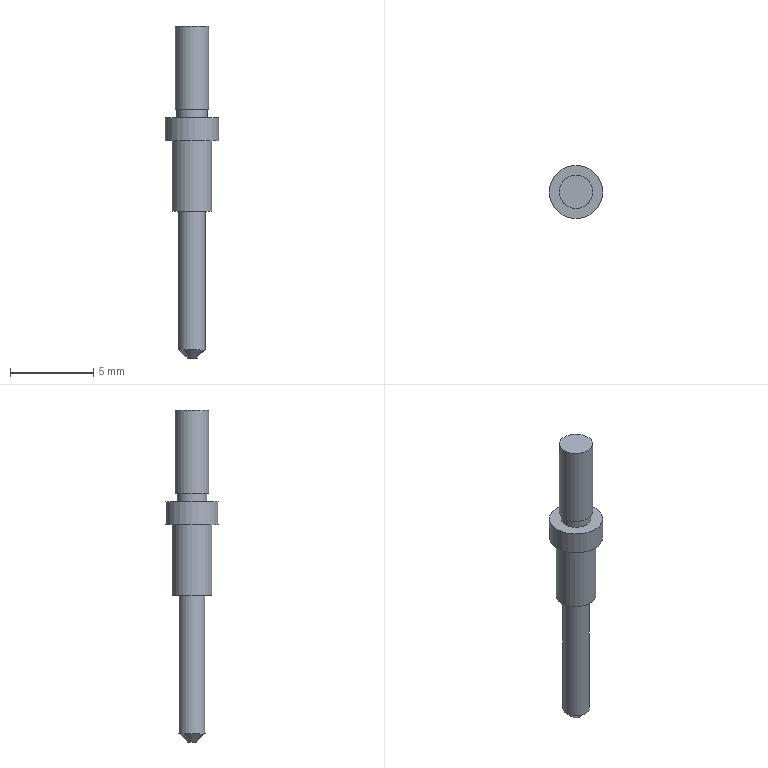Part | STEP file | Radial combiner probe | 1 solid | 12 faces | box 3.2 x 3.2 x 19.92 mm | volume 64.491 mm3 | plane 6 | cylinder 5 | cone 1 | commonest cylinder face diameters 1.6 x1 1.8 x1 2 x1 2.4 x1 3.2 x1
STEP:
#1=CARTESIAN_POINT('',(0.,0.,0.));
#2=DIRECTION('',(0.,0.,1.));
#3=DIRECTION('',(1.,0.,0.));
#4=AXIS2_PLACEMENT_3D('',#1,#2,#3);
#5=CARTESIAN_POINT('',(-216.619,-165.137,75.792));
#6=VERTEX_POINT('',#5);
#7=CARTESIAN_POINT('',(-215.019,-165.137,75.792));
#8=DIRECTION('',(0.,0.,-1.));
#9=DIRECTION('',(-1.,0.,0.));
#10=AXIS2_PLACEMENT_3D('',#7,#8,#9);
#11=CIRCLE('',#10,1.6);
#12=CARTESIAN_POINT('',(-215.019,-165.137,74.402));
#13=DIRECTION('',(0.,0.,1.));
#14=DIRECTION('',(1.,0.,0.));
#15=AXIS2_PLACEMENT_3D('',#12,#13,#14);
#16=CYLINDRICAL_SURFACE('',#15,1.6);
#17=CARTESIAN_POINT('',(9.425,1.39));
#18=DIRECTION('',(-1.,0.));
#19=VECTOR('',#18,1.);
#20=LINE('',#17,#19);
#21=(GEOMETRIC_REPRESENTATION_CONTEXT(2)PARAMETRIC_REPRESENTATION_CONTEXT()REPRESENTATION_CONTEXT('',''));
#22=DEFINITIONAL_REPRESENTATION('',(#20),#21);
#23=PCURVE('',#16,#22);
#24=CARTESIAN_POINT('',(-215.019,-165.137,75.792));
#25=DIRECTION('',(0.,0.,-1.));
#26=DIRECTION('',(-1.,0.,0.));
#27=AXIS2_PLACEMENT_3D('',#24,#25,#26);
#28=PLANE('',#27);
#29=CARTESIAN_POINT('',(0.,0.));
#30=DIRECTION('',(1.,0.));
#31=AXIS2_PLACEMENT_2D('',#29,#30);
#32=CIRCLE('',#31,1.6);
#33=(GEOMETRIC_REPRESENTATION_CONTEXT(2)PARAMETRIC_REPRESENTATION_CONTEXT()REPRESENTATION_CONTEXT('',''));
#34=DEFINITIONAL_REPRESENTATION('',(#32),#33);
#35=PCURVE('',#28,#34);
#36=SURFACE_CURVE('',#11,(#23,#35),.PCURVE_S1.);
#37=EDGE_CURVE('',#6,#6,#36,.T.);
#38=ORIENTED_EDGE('',*,*,#37,.T.);
#39=CARTESIAN_POINT('',(-216.619,-165.137,74.402));
#40=VERTEX_POINT('',#39);
#41=CARTESIAN_POINT('',(-216.619,-165.137,74.402));
#42=CARTESIAN_POINT('',(-216.619,-165.137,75.792));
#43=B_SPLINE_CURVE_WITH_KNOTS('',1,(#41,#42),.UNSPECIFIED.,.F.,.F.,(2,2),(0.,1.39),.PIECEWISE_BEZIER_KNOTS.);
#44=CARTESIAN_POINT('',(3.142,0.));
#45=DIRECTION('',(0.,1.));
#46=VECTOR('',#45,1.);
#47=LINE('',#44,#46);
#48=(GEOMETRIC_REPRESENTATION_CONTEXT(2)PARAMETRIC_REPRESENTATION_CONTEXT()REPRESENTATION_CONTEXT('',''));
#49=DEFINITIONAL_REPRESENTATION('',(#47),#48);
#50=PCURVE('',#16,#49);
#51=CARTESIAN_POINT('',(9.425,0.));
#52=DIRECTION('',(0.,1.));
#53=VECTOR('',#52,1.);
#54=LINE('',#51,#53);
#55=(GEOMETRIC_REPRESENTATION_CONTEXT(2)PARAMETRIC_REPRESENTATION_CONTEXT()REPRESENTATION_CONTEXT('',''));
#56=DEFINITIONAL_REPRESENTATION('',(#54),#55);
#57=PCURVE('',#16,#56);
#58=SEAM_CURVE('',#43,(#50,#57),.PCURVE_S1.);
#59=EDGE_CURVE('',#40,#6,#58,.T.);
#60=ORIENTED_EDGE('',*,*,#59,.F.);
#61=CARTESIAN_POINT('',(-215.019,-165.137,74.402));
#62=DIRECTION('',(0.,0.,-1.));
#63=DIRECTION('',(-1.,0.,0.));
#64=AXIS2_PLACEMENT_3D('',#61,#62,#63);
#65=CIRCLE('',#64,1.6);
#66=CARTESIAN_POINT('',(9.425,0.));
#67=DIRECTION('',(-1.,0.));
#68=VECTOR('',#67,1.);
#69=LINE('',#66,#68);
#70=(GEOMETRIC_REPRESENTATION_CONTEXT(2)PARAMETRIC_REPRESENTATION_CONTEXT()REPRESENTATION_CONTEXT('',''));
#71=DEFINITIONAL_REPRESENTATION('',(#69),#70);
#72=PCURVE('',#16,#71);
#73=CARTESIAN_POINT('',(-215.019,-165.137,74.402));
#74=DIRECTION('',(0.,0.,-1.));
#75=DIRECTION('',(-1.,0.,0.));
#76=AXIS2_PLACEMENT_3D('',#73,#74,#75);
#77=PLANE('',#76);
#78=CARTESIAN_POINT('',(0.,0.));
#79=DIRECTION('',(1.,0.));
#80=AXIS2_PLACEMENT_2D('',#78,#79);
#81=CIRCLE('',#80,1.6);
#82=(GEOMETRIC_REPRESENTATION_CONTEXT(2)PARAMETRIC_REPRESENTATION_CONTEXT()REPRESENTATION_CONTEXT('',''));
#83=DEFINITIONAL_REPRESENTATION('',(#81),#82);
#84=PCURVE('',#77,#83);
#85=SURFACE_CURVE('',#65,(#72,#84),.PCURVE_S1.);
#86=EDGE_CURVE('',#40,#40,#85,.T.);
#87=ORIENTED_EDGE('',*,*,#86,.F.);
#88=ORIENTED_EDGE('',*,*,#59,.T.);
#89=EDGE_LOOP('',(#38,#60,#87,#88));
#90=FACE_BOUND('',#89,.T.);
#91=ADVANCED_FACE('',(#90),#16,.T.);
#92=CARTESIAN_POINT('',(-216.219,-165.137,74.402));
#93=VERTEX_POINT('',#92);
#94=CARTESIAN_POINT('',(-215.019,-165.137,74.402));
#95=DIRECTION('',(0.,0.,-1.));
#96=DIRECTION('',(-1.,0.,0.));
#97=AXIS2_PLACEMENT_3D('',#94,#95,#96);
#98=CIRCLE('',#97,1.2);
#99=CARTESIAN_POINT('',(0.,0.));
#100=DIRECTION('',(1.,0.));
#101=AXIS2_PLACEMENT_2D('',#99,#100);
#102=CIRCLE('',#101,1.2);
#103=(GEOMETRIC_REPRESENTATION_CONTEXT(2)PARAMETRIC_REPRESENTATION_CONTEXT()REPRESENTATION_CONTEXT('',''));
#104=DEFINITIONAL_REPRESENTATION('',(#102),#103);
#105=PCURVE('',#77,#104);
#106=CARTESIAN_POINT('',(-215.019,-165.137,70.172));
#107=DIRECTION('',(0.,0.,1.));
#108=DIRECTION('',(1.,0.,0.));
#109=AXIS2_PLACEMENT_3D('',#106,#107,#108);
#110=CYLINDRICAL_SURFACE('',#109,1.2);
#111=CARTESIAN_POINT('',(9.425,4.23));
#112=DIRECTION('',(-1.,0.));
#113=VECTOR('',#112,1.);
#114=LINE('',#111,#113);
#115=(GEOMETRIC_REPRESENTATION_CONTEXT(2)PARAMETRIC_REPRESENTATION_CONTEXT()REPRESENTATION_CONTEXT('',''));
#116=DEFINITIONAL_REPRESENTATION('',(#114),#115);
#117=PCURVE('',#110,#116);
#118=SURFACE_CURVE('',#98,(#105,#117),.PCURVE_S1.);
#119=EDGE_CURVE('',#93,#93,#118,.T.);
#120=ORIENTED_EDGE('',*,*,#119,.F.);
#121=EDGE_LOOP('',(#120));
#122=FACE_BOUND('',#121,.T.);
#123=ORIENTED_EDGE('',*,*,#86,.T.);
#124=EDGE_LOOP('',(#123));
#125=FACE_BOUND('',#124,.T.);
#126=ADVANCED_FACE('',(#122,#125),#77,.T.);
#127=CARTESIAN_POINT('',(-214.119,-165.137,75.792));
#128=VERTEX_POINT('',#127);
#129=CARTESIAN_POINT('',(-215.019,-165.137,75.792));
#130=DIRECTION('',(0.,0.,1.));
#131=DIRECTION('',(1.,0.,0.));
#132=AXIS2_PLACEMENT_3D('',#129,#130,#131);
#133=CIRCLE('',#132,0.9);
#134=CARTESIAN_POINT('',(-0.9,0.));
#135=CARTESIAN_POINT('',(-0.9,1.559));
#136=CARTESIAN_POINT('',(0.45,0.7794));
#137=CARTESIAN_POINT('',(1.8,0.));
#138=CARTESIAN_POINT('',(0.45,-0.7794));
#139=CARTESIAN_POINT('',(-0.9,-1.559));
#140=CARTESIAN_POINT('',(-0.9,0.));
#141=(BOUNDED_CURVE()B_SPLINE_CURVE(2,(#134,#135,#136,#137,#138,#139,#140),.UNSPECIFIED.,.T.,.F.)B_SPLINE_CURVE_WITH_KNOTS((1,2,2,2,2,1),(-2.094,0.,2.094,4.189,6.283,8.378),.UNSPECIFIED.)CURVE()GEOMETRIC_REPRESENTATION_ITEM()RATIONAL_B_SPLINE_CURVE((1.,0.5,1.,0.5,1.,0.5,1.))REPRESENTATION_ITEM(''));
#142=(GEOMETRIC_REPRESENTATION_CONTEXT(2)PARAMETRIC_REPRESENTATION_CONTEXT()REPRESENTATION_CONTEXT('',''));
#143=DEFINITIONAL_REPRESENTATION('',(#141),#142);
#144=PCURVE('',#28,#143);
#145=CARTESIAN_POINT('',(-215.019,-165.137,76.292));
#146=DIRECTION('',(0.,0.,-1.));
#147=DIRECTION('',(-1.,0.,0.));
#148=AXIS2_PLACEMENT_3D('',#145,#146,#147);
#149=CYLINDRICAL_SURFACE('',#148,0.9);
#150=CARTESIAN_POINT('',(9.425,0.5));
#151=DIRECTION('',(-1.,0.));
#152=VECTOR('',#151,1.);
#153=LINE('',#150,#152);
#154=(GEOMETRIC_REPRESENTATION_CONTEXT(2)PARAMETRIC_REPRESENTATION_CONTEXT()REPRESENTATION_CONTEXT('',''));
#155=DEFINITIONAL_REPRESENTATION('',(#153),#154);
#156=PCURVE('',#149,#155);
#157=SURFACE_CURVE('',#133,(#144,#156),.PCURVE_S1.);
#158=EDGE_CURVE('',#128,#128,#157,.T.);
#159=ORIENTED_EDGE('',*,*,#158,.F.);
#160=EDGE_LOOP('',(#159));
#161=FACE_BOUND('',#160,.T.);
#162=ORIENTED_EDGE('',*,*,#37,.F.);
#163=EDGE_LOOP('',(#162));
#164=FACE_BOUND('',#163,.T.);
#165=ADVANCED_FACE('',(#161,#164),#28,.F.);
#166=ORIENTED_EDGE('',*,*,#119,.T.);
#167=CARTESIAN_POINT('',(-216.219,-165.137,70.172));
#168=VERTEX_POINT('',#167);
#169=CARTESIAN_POINT('',(-216.219,-165.137,70.172));
#170=CARTESIAN_POINT('',(-216.219,-165.137,74.402));
#171=B_SPLINE_CURVE_WITH_KNOTS('',1,(#169,#170),.UNSPECIFIED.,.F.,.F.,(2,2),(0.,4.23),.PIECEWISE_BEZIER_KNOTS.);
#172=CARTESIAN_POINT('',(3.142,0.));
#173=DIRECTION('',(0.,1.));
#174=VECTOR('',#173,1.);
#175=LINE('',#172,#174);
#176=(GEOMETRIC_REPRESENTATION_CONTEXT(2)PARAMETRIC_REPRESENTATION_CONTEXT()REPRESENTATION_CONTEXT('',''));
#177=DEFINITIONAL_REPRESENTATION('',(#175),#176);
#178=PCURVE('',#110,#177);
#179=CARTESIAN_POINT('',(9.425,0.));
#180=DIRECTION('',(0.,1.));
#181=VECTOR('',#180,1.);
#182=LINE('',#179,#181);
#183=(GEOMETRIC_REPRESENTATION_CONTEXT(2)PARAMETRIC_REPRESENTATION_CONTEXT()REPRESENTATION_CONTEXT('',''));
#184=DEFINITIONAL_REPRESENTATION('',(#182),#183);
#185=PCURVE('',#110,#184);
#186=SEAM_CURVE('',#171,(#178,#185),.PCURVE_S1.);
#187=EDGE_CURVE('',#168,#93,#186,.T.);
#188=ORIENTED_EDGE('',*,*,#187,.F.);
#189=CARTESIAN_POINT('',(-215.019,-165.137,70.172));
#190=DIRECTION('',(0.,0.,-1.));
#191=DIRECTION('',(-1.,0.,0.));
#192=AXIS2_PLACEMENT_3D('',#189,#190,#191);
#193=CIRCLE('',#192,1.2);
#194=CARTESIAN_POINT('',(9.425,0.));
#195=DIRECTION('',(-1.,0.));
#196=VECTOR('',#195,1.);
#197=LINE('',#194,#196);
#198=(GEOMETRIC_REPRESENTATION_CONTEXT(2)PARAMETRIC_REPRESENTATION_CONTEXT()REPRESENTATION_CONTEXT('',''));
#199=DEFINITIONAL_REPRESENTATION('',(#197),#198);
#200=PCURVE('',#110,#199);
#201=CARTESIAN_POINT('',(-215.019,-165.137,70.172));
#202=DIRECTION('',(0.,0.,-1.));
#203=DIRECTION('',(-1.,0.,0.));
#204=AXIS2_PLACEMENT_3D('',#201,#202,#203);
#205=PLANE('',#204);
#206=CARTESIAN_POINT('',(0.,0.));
#207=DIRECTION('',(1.,0.));
#208=AXIS2_PLACEMENT_2D('',#206,#207);
#209=CIRCLE('',#208,1.2);
#210=(GEOMETRIC_REPRESENTATION_CONTEXT(2)PARAMETRIC_REPRESENTATION_CONTEXT()REPRESENTATION_CONTEXT('',''));
#211=DEFINITIONAL_REPRESENTATION('',(#209),#210);
#212=PCURVE('',#205,#211);
#213=SURFACE_CURVE('',#193,(#200,#212),.PCURVE_S1.);
#214=EDGE_CURVE('',#168,#168,#213,.T.);
#215=ORIENTED_EDGE('',*,*,#214,.F.);
#216=ORIENTED_EDGE('',*,*,#187,.T.);
#217=EDGE_LOOP('',(#166,#188,#215,#216));
#218=FACE_BOUND('',#217,.T.);
#219=ADVANCED_FACE('',(#218),#110,.T.);
#220=CARTESIAN_POINT('',(-215.819,-165.137,70.172));
#221=VERTEX_POINT('',#220);
#222=CARTESIAN_POINT('',(-215.019,-165.137,70.172));
#223=DIRECTION('',(0.,0.,-1.));
#224=DIRECTION('',(-1.,0.,0.));
#225=AXIS2_PLACEMENT_3D('',#222,#223,#224);
#226=CIRCLE('',#225,0.8);
#227=CARTESIAN_POINT('',(0.,0.));
#228=DIRECTION('',(1.,0.));
#229=AXIS2_PLACEMENT_2D('',#227,#228);
#230=CIRCLE('',#229,0.8);
#231=(GEOMETRIC_REPRESENTATION_CONTEXT(2)PARAMETRIC_REPRESENTATION_CONTEXT()REPRESENTATION_CONTEXT('',''));
#232=DEFINITIONAL_REPRESENTATION('',(#230),#231);
#233=PCURVE('',#205,#232);
#234=CARTESIAN_POINT('',(-215.019,-165.137,61.372));
#235=DIRECTION('',(0.,0.,1.));
#236=DIRECTION('',(1.,0.,0.));
#237=AXIS2_PLACEMENT_3D('',#234,#235,#236);
#238=CYLINDRICAL_SURFACE('',#237,0.8);
#239=CARTESIAN_POINT('',(9.425,8.8));
#240=DIRECTION('',(-1.,0.));
#241=VECTOR('',#240,1.);
#242=LINE('',#239,#241);
#243=(GEOMETRIC_REPRESENTATION_CONTEXT(2)PARAMETRIC_REPRESENTATION_CONTEXT()REPRESENTATION_CONTEXT('',''));
#244=DEFINITIONAL_REPRESENTATION('',(#242),#243);
#245=PCURVE('',#238,#244);
#246=SURFACE_CURVE('',#226,(#233,#245),.PCURVE_S1.);
#247=EDGE_CURVE('',#221,#221,#246,.T.);
#248=ORIENTED_EDGE('',*,*,#247,.F.);
#249=EDGE_LOOP('',(#248));
#250=FACE_BOUND('',#249,.T.);
#251=ORIENTED_EDGE('',*,*,#214,.T.);
#252=EDGE_LOOP('',(#251));
#253=FACE_BOUND('',#252,.T.);
#254=ADVANCED_FACE('',(#250,#253),#205,.T.);
#255=CARTESIAN_POINT('',(-215.819,-165.137,61.872));
#256=VERTEX_POINT('',#255);
#257=CARTESIAN_POINT('',(-215.019,-165.137,61.872));
#258=DIRECTION('',(0.,0.,1.));
#259=DIRECTION('',(-1.,0.,0.));
#260=AXIS2_PLACEMENT_3D('',#257,#258,#259);
#261=CIRCLE('',#260,0.8);
#262=CARTESIAN_POINT('',(3.142,0.5));
#263=DIRECTION('',(1.,0.));
#264=VECTOR('',#263,1.);
#265=LINE('',#262,#264);
#266=(GEOMETRIC_REPRESENTATION_CONTEXT(2)PARAMETRIC_REPRESENTATION_CONTEXT()REPRESENTATION_CONTEXT('',''));
#267=DEFINITIONAL_REPRESENTATION('',(#265),#266);
#268=PCURVE('',#238,#267);
#269=CARTESIAN_POINT('',(-215.019,-165.137,61.372));
#270=DIRECTION('',(0.,0.,1.));
#271=DIRECTION('',(1.,0.,0.));
#272=AXIS2_PLACEMENT_3D('',#269,#270,#271);
#273=CONICAL_SURFACE('',#272,0.3,0.7854);
#274=CARTESIAN_POINT('',(3.142,0.5));
#275=DIRECTION('',(1.,0.));
#276=VECTOR('',#275,1.);
#277=LINE('',#274,#276);
#278=(GEOMETRIC_REPRESENTATION_CONTEXT(2)PARAMETRIC_REPRESENTATION_CONTEXT()REPRESENTATION_CONTEXT('',''));
#279=DEFINITIONAL_REPRESENTATION('',(#277),#278);
#280=PCURVE('',#273,#279);
#281=SURFACE_CURVE('',#261,(#268,#280),.PCURVE_S1.);
#282=EDGE_CURVE('',#256,#256,#281,.T.);
#283=ORIENTED_EDGE('',*,*,#282,.T.);
#284=CARTESIAN_POINT('',(-215.819,-165.137,61.872));
#285=CARTESIAN_POINT('',(-215.819,-165.137,70.172));
#286=B_SPLINE_CURVE_WITH_KNOTS('',1,(#284,#285),.UNSPECIFIED.,.F.,.F.,(2,2),(0.5,8.8),.PIECEWISE_BEZIER_KNOTS.);
#287=CARTESIAN_POINT('',(9.425,0.));
#288=DIRECTION('',(0.,1.));
#289=VECTOR('',#288,1.);
#290=LINE('',#287,#289);
#291=(GEOMETRIC_REPRESENTATION_CONTEXT(2)PARAMETRIC_REPRESENTATION_CONTEXT()REPRESENTATION_CONTEXT('',''));
#292=DEFINITIONAL_REPRESENTATION('',(#290),#291);
#293=PCURVE('',#238,#292);
#294=CARTESIAN_POINT('',(3.142,0.));
#295=DIRECTION('',(0.,1.));
#296=VECTOR('',#295,1.);
#297=LINE('',#294,#296);
#298=(GEOMETRIC_REPRESENTATION_CONTEXT(2)PARAMETRIC_REPRESENTATION_CONTEXT()REPRESENTATION_CONTEXT('',''));
#299=DEFINITIONAL_REPRESENTATION('',(#297),#298);
#300=PCURVE('',#238,#299);
#301=SEAM_CURVE('',#286,(#293,#300),.PCURVE_S1.);
#302=EDGE_CURVE('',#256,#221,#301,.T.);
#303=ORIENTED_EDGE('',*,*,#302,.T.);
#304=ORIENTED_EDGE('',*,*,#247,.T.);
#305=ORIENTED_EDGE('',*,*,#302,.F.);
#306=EDGE_LOOP('',(#283,#303,#304,#305));
#307=FACE_BOUND('',#306,.T.);
#308=ADVANCED_FACE('',(#307),#238,.T.);
#309=CARTESIAN_POINT('',(-215.319,-165.137,61.372));
#310=VERTEX_POINT('',#309);
#311=CARTESIAN_POINT('',(-215.019,-165.137,61.372));
#312=DIRECTION('',(0.,0.,-1.));
#313=DIRECTION('',(-1.,0.,0.));
#314=AXIS2_PLACEMENT_3D('',#311,#312,#313);
#315=CIRCLE('',#314,0.3);
#316=CARTESIAN_POINT('',(-215.019,-165.137,61.372));
#317=DIRECTION('',(0.,0.,-1.));
#318=DIRECTION('',(-1.,0.,0.));
#319=AXIS2_PLACEMENT_3D('',#316,#317,#318);
#320=PLANE('',#319);
#321=CARTESIAN_POINT('',(0.,0.));
#322=DIRECTION('',(1.,0.));
#323=AXIS2_PLACEMENT_2D('',#321,#322);
#324=CIRCLE('',#323,0.3);
#325=(GEOMETRIC_REPRESENTATION_CONTEXT(2)PARAMETRIC_REPRESENTATION_CONTEXT()REPRESENTATION_CONTEXT('',''));
#326=DEFINITIONAL_REPRESENTATION('',(#324),#325);
#327=PCURVE('',#320,#326);
#328=CARTESIAN_POINT('',(9.425,0.));
#329=DIRECTION('',(-1.,0.));
#330=VECTOR('',#329,1.);
#331=LINE('',#328,#330);
#332=(GEOMETRIC_REPRESENTATION_CONTEXT(2)PARAMETRIC_REPRESENTATION_CONTEXT()REPRESENTATION_CONTEXT('',''));
#333=DEFINITIONAL_REPRESENTATION('',(#331),#332);
#334=PCURVE('',#273,#333);
#335=SURFACE_CURVE('',#315,(#327,#334),.PCURVE_S1.);
#336=EDGE_CURVE('',#310,#310,#335,.T.);
#337=ORIENTED_EDGE('',*,*,#336,.T.);
#338=EDGE_LOOP('',(#337));
#339=FACE_BOUND('',#338,.T.);
#340=ADVANCED_FACE('',(#339),#320,.T.);
#341=CARTESIAN_POINT('',(-214.119,-165.137,76.292));
#342=VERTEX_POINT('',#341);
#343=CARTESIAN_POINT('',(-215.019,-165.137,76.292));
#344=DIRECTION('',(0.,0.,1.));
#345=DIRECTION('',(1.,0.,0.));
#346=AXIS2_PLACEMENT_3D('',#343,#344,#345);
#347=CIRCLE('',#346,0.9);
#348=CARTESIAN_POINT('',(9.425,0.));
#349=DIRECTION('',(-1.,0.));
#350=VECTOR('',#349,1.);
#351=LINE('',#348,#350);
#352=(GEOMETRIC_REPRESENTATION_CONTEXT(2)PARAMETRIC_REPRESENTATION_CONTEXT()REPRESENTATION_CONTEXT('',''));
#353=DEFINITIONAL_REPRESENTATION('',(#351),#352);
#354=PCURVE('',#149,#353);
#355=CARTESIAN_POINT('',(-215.019,-165.137,76.292));
#356=DIRECTION('',(0.,0.,1.));
#357=DIRECTION('',(1.,0.,0.));
#358=AXIS2_PLACEMENT_3D('',#355,#356,#357);
#359=PLANE('',#358);
#360=CARTESIAN_POINT('',(0.,0.));
#361=DIRECTION('',(1.,0.));
#362=AXIS2_PLACEMENT_2D('',#360,#361);
#363=CIRCLE('',#362,0.9);
#364=(GEOMETRIC_REPRESENTATION_CONTEXT(2)PARAMETRIC_REPRESENTATION_CONTEXT()REPRESENTATION_CONTEXT('',''));
#365=DEFINITIONAL_REPRESENTATION('',(#363),#364);
#366=PCURVE('',#359,#365);
#367=SURFACE_CURVE('',#347,(#354,#366),.PCURVE_S1.);
#368=EDGE_CURVE('',#342,#342,#367,.T.);
#369=ORIENTED_EDGE('',*,*,#368,.F.);
#370=CARTESIAN_POINT('',(-214.119,-165.137,76.292));
#371=CARTESIAN_POINT('',(-214.119,-165.137,75.792));
#372=B_SPLINE_CURVE_WITH_KNOTS('',1,(#370,#371),.UNSPECIFIED.,.F.,.F.,(2,2),(0.,0.5),.PIECEWISE_BEZIER_KNOTS.);
#373=CARTESIAN_POINT('',(9.425,0.));
#374=DIRECTION('',(0.,1.));
#375=VECTOR('',#374,1.);
#376=LINE('',#373,#375);
#377=(GEOMETRIC_REPRESENTATION_CONTEXT(2)PARAMETRIC_REPRESENTATION_CONTEXT()REPRESENTATION_CONTEXT('',''));
#378=DEFINITIONAL_REPRESENTATION('',(#376),#377);
#379=PCURVE('',#149,#378);
#380=CARTESIAN_POINT('',(3.142,0.));
#381=DIRECTION('',(0.,1.));
#382=VECTOR('',#381,1.);
#383=LINE('',#380,#382);
#384=(GEOMETRIC_REPRESENTATION_CONTEXT(2)PARAMETRIC_REPRESENTATION_CONTEXT()REPRESENTATION_CONTEXT('',''));
#385=DEFINITIONAL_REPRESENTATION('',(#383),#384);
#386=PCURVE('',#149,#385);
#387=SEAM_CURVE('',#372,(#379,#386),.PCURVE_S1.);
#388=EDGE_CURVE('',#342,#128,#387,.T.);
#389=ORIENTED_EDGE('',*,*,#388,.T.);
#390=ORIENTED_EDGE('',*,*,#158,.T.);
#391=ORIENTED_EDGE('',*,*,#388,.F.);
#392=EDGE_LOOP('',(#369,#389,#390,#391));
#393=FACE_BOUND('',#392,.T.);
#394=ADVANCED_FACE('',(#393),#149,.T.);
#395=CARTESIAN_POINT('',(-214.019,-165.137,81.292));
#396=VERTEX_POINT('',#395);
#397=CARTESIAN_POINT('',(-215.019,-165.137,81.292));
#398=DIRECTION('',(0.,0.,1.));
#399=DIRECTION('',(1.,0.,0.));
#400=AXIS2_PLACEMENT_3D('',#397,#398,#399);
#401=CIRCLE('',#400,1.);
#402=CARTESIAN_POINT('',(-215.019,-165.137,81.292));
#403=DIRECTION('',(0.,0.,-1.));
#404=DIRECTION('',(-1.,0.,0.));
#405=AXIS2_PLACEMENT_3D('',#402,#403,#404);
#406=CYLINDRICAL_SURFACE('',#405,1.);
#407=CARTESIAN_POINT('',(9.425,0.));
#408=DIRECTION('',(-1.,0.));
#409=VECTOR('',#408,1.);
#410=LINE('',#407,#409);
#411=(GEOMETRIC_REPRESENTATION_CONTEXT(2)PARAMETRIC_REPRESENTATION_CONTEXT()REPRESENTATION_CONTEXT('',''));
#412=DEFINITIONAL_REPRESENTATION('',(#410),#411);
#413=PCURVE('',#406,#412);
#414=CARTESIAN_POINT('',(-215.019,-165.137,81.292));
#415=DIRECTION('',(0.,0.,1.));
#416=DIRECTION('',(1.,0.,0.));
#417=AXIS2_PLACEMENT_3D('',#414,#415,#416);
#418=PLANE('',#417);
#419=CARTESIAN_POINT('',(0.,0.));
#420=DIRECTION('',(1.,0.));
#421=AXIS2_PLACEMENT_2D('',#419,#420);
#422=CIRCLE('',#421,1.);
#423=(GEOMETRIC_REPRESENTATION_CONTEXT(2)PARAMETRIC_REPRESENTATION_CONTEXT()REPRESENTATION_CONTEXT('',''));
#424=DEFINITIONAL_REPRESENTATION('',(#422),#423);
#425=PCURVE('',#418,#424);
#426=SURFACE_CURVE('',#401,(#413,#425),.PCURVE_S1.);
#427=EDGE_CURVE('',#396,#396,#426,.T.);
#428=ORIENTED_EDGE('',*,*,#427,.F.);
#429=CARTESIAN_POINT('',(-214.019,-165.137,76.292));
#430=VERTEX_POINT('',#429);
#431=CARTESIAN_POINT('',(-214.019,-165.137,81.292));
#432=CARTESIAN_POINT('',(-214.019,-165.137,76.292));
#433=B_SPLINE_CURVE_WITH_KNOTS('',1,(#431,#432),.UNSPECIFIED.,.F.,.F.,(2,2),(0.,5.),.PIECEWISE_BEZIER_KNOTS.);
#434=CARTESIAN_POINT('',(9.425,0.));
#435=DIRECTION('',(0.,1.));
#436=VECTOR('',#435,1.);
#437=LINE('',#434,#436);
#438=(GEOMETRIC_REPRESENTATION_CONTEXT(2)PARAMETRIC_REPRESENTATION_CONTEXT()REPRESENTATION_CONTEXT('',''));
#439=DEFINITIONAL_REPRESENTATION('',(#437),#438);
#440=PCURVE('',#406,#439);
#441=CARTESIAN_POINT('',(3.142,0.));
#442=DIRECTION('',(0.,1.));
#443=VECTOR('',#442,1.);
#444=LINE('',#441,#443);
#445=(GEOMETRIC_REPRESENTATION_CONTEXT(2)PARAMETRIC_REPRESENTATION_CONTEXT()REPRESENTATION_CONTEXT('',''));
#446=DEFINITIONAL_REPRESENTATION('',(#444),#445);
#447=PCURVE('',#406,#446);
#448=SEAM_CURVE('',#433,(#440,#447),.PCURVE_S1.);
#449=EDGE_CURVE('',#396,#430,#448,.T.);
#450=ORIENTED_EDGE('',*,*,#449,.T.);
#451=CARTESIAN_POINT('',(-215.019,-165.137,76.292));
#452=DIRECTION('',(0.,0.,1.));
#453=DIRECTION('',(1.,0.,0.));
#454=AXIS2_PLACEMENT_3D('',#451,#452,#453);
#455=CIRCLE('',#454,1.);
#456=CARTESIAN_POINT('',(9.425,5.));
#457=DIRECTION('',(-1.,0.));
#458=VECTOR('',#457,1.);
#459=LINE('',#456,#458);
#460=(GEOMETRIC_REPRESENTATION_CONTEXT(2)PARAMETRIC_REPRESENTATION_CONTEXT()REPRESENTATION_CONTEXT('',''));
#461=DEFINITIONAL_REPRESENTATION('',(#459),#460);
#462=PCURVE('',#406,#461);
#463=CARTESIAN_POINT('',(0.,0.));
#464=DIRECTION('',(1.,0.));
#465=AXIS2_PLACEMENT_2D('',#463,#464);
#466=CIRCLE('',#465,1.);
#467=(GEOMETRIC_REPRESENTATION_CONTEXT(2)PARAMETRIC_REPRESENTATION_CONTEXT()REPRESENTATION_CONTEXT('',''));
#468=DEFINITIONAL_REPRESENTATION('',(#466),#467);
#469=PCURVE('',#359,#468);
#470=SURFACE_CURVE('',#455,(#462,#469),.PCURVE_S1.);
#471=EDGE_CURVE('',#430,#430,#470,.T.);
#472=ORIENTED_EDGE('',*,*,#471,.T.);
#473=ORIENTED_EDGE('',*,*,#449,.F.);
#474=EDGE_LOOP('',(#428,#450,#472,#473));
#475=FACE_BOUND('',#474,.T.);
#476=ADVANCED_FACE('',(#475),#406,.T.);
#477=ORIENTED_EDGE('',*,*,#427,.T.);
#478=EDGE_LOOP('',(#477));
#479=FACE_BOUND('',#478,.T.);
#480=ADVANCED_FACE('',(#479),#418,.T.);
#481=ORIENTED_EDGE('',*,*,#368,.T.);
#482=EDGE_LOOP('',(#481));
#483=FACE_BOUND('',#482,.T.);
#484=ORIENTED_EDGE('',*,*,#471,.F.);
#485=EDGE_LOOP('',(#484));
#486=FACE_BOUND('',#485,.T.);
#487=ADVANCED_FACE('',(#483,#486),#359,.F.);
#488=ORIENTED_EDGE('',*,*,#282,.F.);
#489=CARTESIAN_POINT('',(-215.319,-165.137,61.372));
#490=CARTESIAN_POINT('',(-215.819,-165.137,61.872));
#491=B_SPLINE_CURVE_WITH_KNOTS('',1,(#489,#490),.UNSPECIFIED.,.F.,.F.,(2,2),(0.,0.7071),.PIECEWISE_BEZIER_KNOTS.);
#492=CARTESIAN_POINT('',(3.142,0.));
#493=DIRECTION('',(0.,1.));
#494=VECTOR('',#493,1.);
#495=LINE('',#492,#494);
#496=(GEOMETRIC_REPRESENTATION_CONTEXT(2)PARAMETRIC_REPRESENTATION_CONTEXT()REPRESENTATION_CONTEXT('',''));
#497=DEFINITIONAL_REPRESENTATION('',(#495),#496);
#498=PCURVE('',#273,#497);
#499=CARTESIAN_POINT('',(9.425,0.));
#500=DIRECTION('',(0.,1.));
#501=VECTOR('',#500,1.);
#502=LINE('',#499,#501);
#503=(GEOMETRIC_REPRESENTATION_CONTEXT(2)PARAMETRIC_REPRESENTATION_CONTEXT()REPRESENTATION_CONTEXT('',''));
#504=DEFINITIONAL_REPRESENTATION('',(#502),#503);
#505=PCURVE('',#273,#504);
#506=SEAM_CURVE('',#491,(#498,#505),.PCURVE_S1.);
#507=EDGE_CURVE('',#310,#256,#506,.T.);
#508=ORIENTED_EDGE('',*,*,#507,.F.);
#509=ORIENTED_EDGE('',*,*,#336,.F.);
#510=ORIENTED_EDGE('',*,*,#507,.T.);
#511=EDGE_LOOP('',(#488,#508,#509,#510));
#512=FACE_BOUND('',#511,.T.);
#513=ADVANCED_FACE('',(#512),#273,.T.);
#514=CLOSED_SHELL('',(#91,#126,#165,#219,#254,#308,#340,#394,#476,#480,#487,#513));
#515=MANIFOLD_SOLID_BREP('',#514);
#516=(LENGTH_UNIT()NAMED_UNIT(*)SI_UNIT(.MILLI.,.METRE.));
#517=UNCERTAINTY_MEASURE_WITH_UNIT(LENGTH_MEASURE(0.00001),#516,'','');
#518=(NAMED_UNIT(*)PLANE_ANGLE_UNIT()SI_UNIT($,.RADIAN.));
#519=(NAMED_UNIT(*)SI_UNIT($,.STERADIAN.)SOLID_ANGLE_UNIT());
#520=(GEOMETRIC_REPRESENTATION_CONTEXT(3)GLOBAL_UNCERTAINTY_ASSIGNED_CONTEXT((#517))GLOBAL_UNIT_ASSIGNED_CONTEXT((#516,#518,#519))REPRESENTATION_CONTEXT('',''));
#521=ADVANCED_BREP_SHAPE_REPRESENTATION('',(#4,#515),#520);